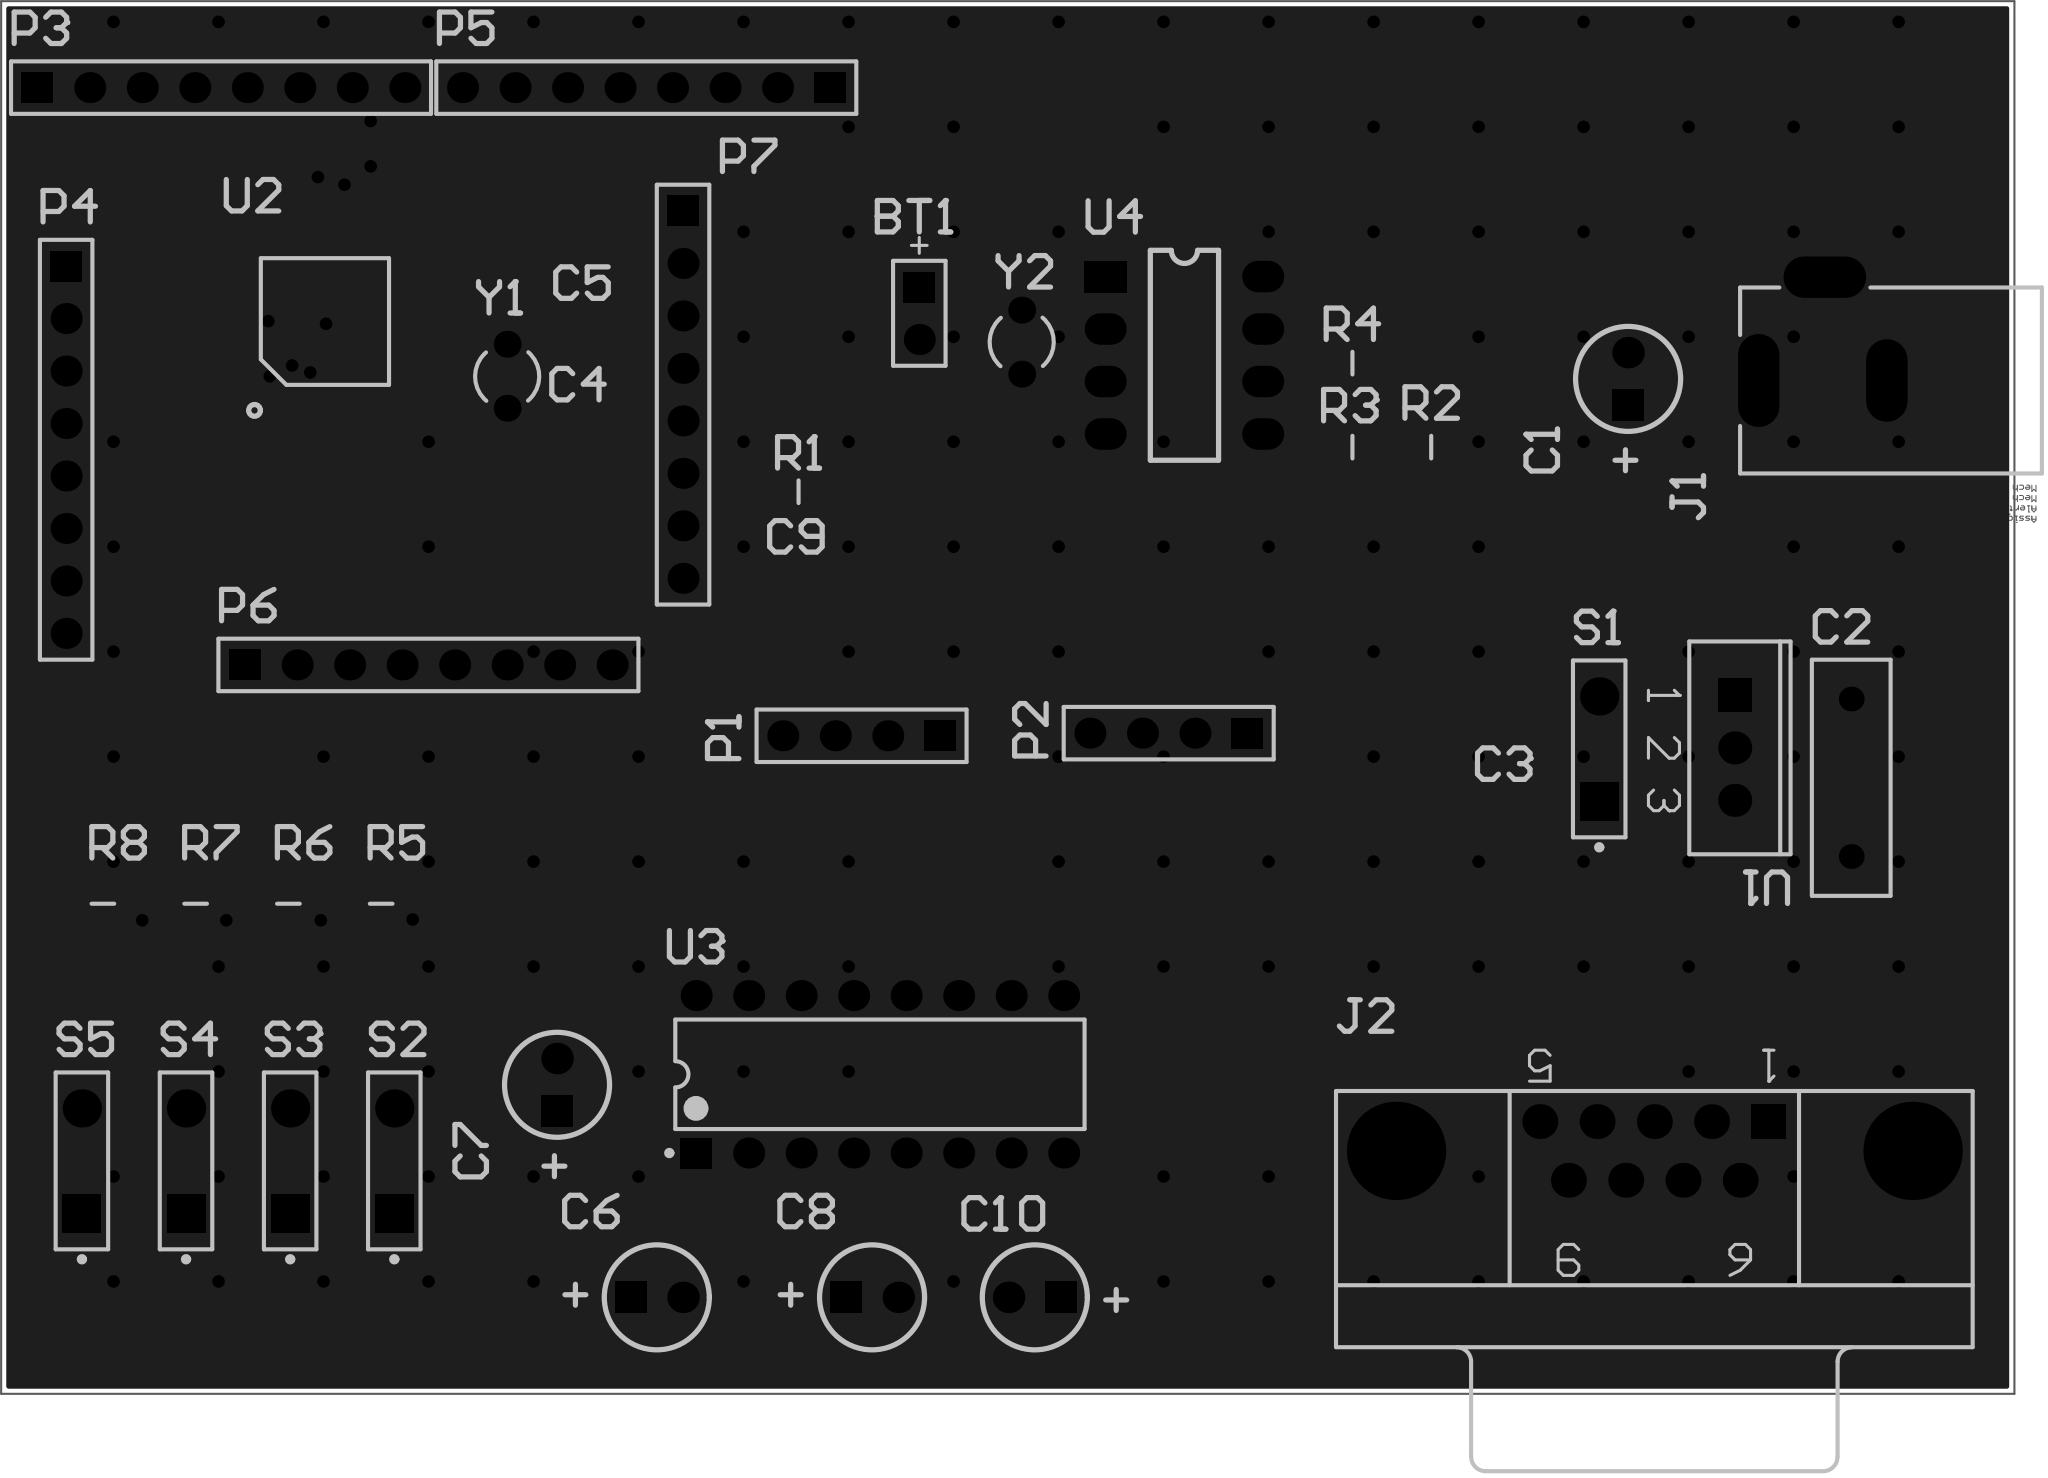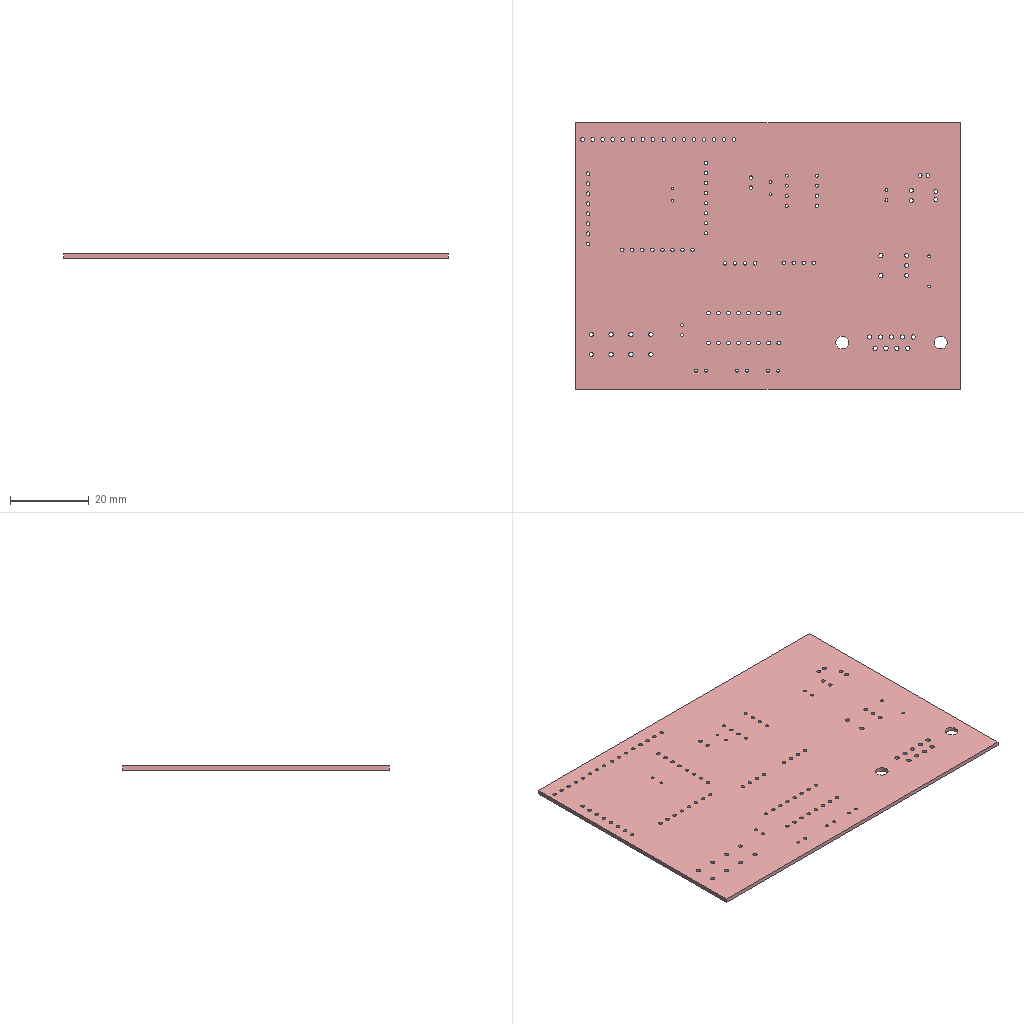Circuit board layout | Altium Designer | box 97.4 x 67.4 x 1.1 mm
Layer stack:
# Altium Designer layer stack of  (unit mm; dielectric type: 0 none, 1 core, 2 prepreg, 3 surface material)
index,name,kind,layer,copper_thickness_mm,dielectric_type,dielectric_thickness_mm,dielectric_material,dielectric_constant
0,Top Paste Mask Layer,other,,,,,,
1,Top Silkscreen Layer,other,,,,,,
2,Top Solder Mask Layer,dielectric,,,3,0.0102,Solder Resist,3.5
3,Top Layer,copper,Top Layer,0.0356,,,,
4,SUBSTRATE1,dielectric,,,3,0.32,FR-4,4.8
5,SUBSTRATE2,dielectric,,,3,0.32,FR-4,4.8
6,SUBSTRATE3,dielectric,,,3,0.32,FR-4,4.8
7,Bottom Layer,copper,Bottom Layer,0.0356,,,,
8,Bottom Solder Mask Layer,dielectric,,,3,0.0102,Solder Resist,3.5
9,Bottom Silkscreen Layer,other,,,,,,
10,Bottom Paste Mask Layer,other,,,,,,
# drill layer pairs: low layer,high layer
drill_pair,Top Layer,Bottom Layer
Part placement:
Designator,Comment,Layer,Footprint,Center-X(mm),Center-Y(mm),Rotation
Y2,XTAL,TopLayer,R38,130.937,136.652,180
Y1,XTAL,TopLayer,R38,106.045,135.001,0
U4,DS1302,TopLayer,DIP-8,138.811,136.017,0
U3,MAX232ACPE,TopLayer,PE16A,124.079,101.219,90
U2,STC12C5A60S2,TopLayer,TQFP-44,97.302,137.696,0
U1,MC7805BT,TopLayer,221A-04,165.434,117.017,270
S5,SW-PB,TopLayer,SPST-2,85.471,97.028,90
S4,SW-PB,TopLayer,SPST-2,90.509,97.028,90
S3,SW-PB,TopLayer,SPST-2,95.546,97.028,90
S2,SW-PB,TopLayer,SPST-2,100.584,97.028,90
S1,SW-SPST,TopLayer,SPST-2,158.877,116.967,90
R8,Res2,TopLayer,6-0805_L,86.487,109.474,90
R7,Res2,TopLayer,6-0805_L,90.974,109.474,90
R6,Res2,TopLayer,6-0805_L,95.462,109.474,90
R5,Res2,TopLayer,6-0805_L,99.949,109.474,90
R4,Res2,TopLayer,6-0805_L,146.939,135.636,180
R3,Res2,TopLayer,6-0805_L,146.939,131.572,0
R2,Res2,TopLayer,6-0805_L,150.749,131.572,180
R1,Res2,TopLayer,6-0805_L,120.142,129.413,180
P7,PIN4,TopLayer,HDR1X8,114.554,134.112,270
P6,PIN3,TopLayer,HDR1X8,102.235,121.031,0
P5,PIN2,TopLayer,HDR1X8,112.776,148.971,180
P4,PIN1,TopLayer,HDR1X8,84.709,131.445,270
P3,PIN0,TopLayer,HDR1X8,92.202,148.971,0
P2,POWER,TopLayer,HDR1X4,138.049,117.729,180
P1,DEBUG,TopLayer,HDR1X4,123.19,117.602,180
J2,D Connector 9,TopLayer,DSUB1.385-2H9,161.544,97.511,180
J1,PWR2.5,TopLayer,KLD-0202,169.693,136.672,180
C10,Cap Pol1,TopLayer,RB2.54-5.08,131.572,90.424,180
C9,Cap,TopLayer,C0805,120.015,125.095,0
C8,Cap Pol1,TopLayer,RB2.54-5.08,123.698,90.424,0
C7,Cap Pol1,TopLayer,RB2.54-5.08,108.458,100.711,90
C6,Cap Pol1,TopLayer,RB2.54-5.08,113.284,90.424,0
C5,Cap,TopLayer,C0805,109.601,137.16,0
C4,Cap,TopLayer,C0805,109.474,132.461,0
C3,Cap,TopLayer,C0805,154.385,114.477,0
C2,Cap,TopLayer,RAD-0.3,171.069,115.57,90
C1,Cap Pol1,TopLayer,RB2.54-5.08,160.274,134.874,90
BT1,Battery,TopLayer,BAT-2,125.984,138.049,270
Pad and via stacks:
# Altium Designer via and pad stacks of  (unit mm). Each distinct definition once, with the count of objects using it.
# via: kind,start_layer,end_layer,hole_mm,diameter_mm,mode(0 simple;1 top-mid-bottom;2 full stack),diameter_per_layer,count,example_net
# pad: kind,layer,hole_mm,hole_type(0 round;1 square;2 slot),plating,top_size,top_shape(1 round;2 rect;3 octagon;9 rounded rect),mid_size,bottom_size,mode,footprint,size_per_layer,count,example
pad,Multi-Layer,0.7,0,plated,1.3x1.3,1,1.3x1.3,1.3x1.3,0,R38,,4,Y2.1
pad,Multi-Layer,0.8128,0,plated,2.032x1.524,1,2.032x1.524,2.032x1.524,0,DIP-8,,7,U4.3
pad,Multi-Layer,0.8128,0,plated,2.032x1.524,2,2.032x1.524,2.032x1.524,0,DIP-8,,1,U4.1
pad,Multi-Layer,0.9,0,plated,1.5x1.5,1,1.5x1.5,1.5x1.5,0,PE16A,,15,U3.9
pad,Multi-Layer,0.9,0,plated,1.5x1.5,2,1.5x1.5,1.5x1.5,0,PE16A,,1,U3.1
pad,Multi-Layer,1,0,plated,1.6x1.6,2,1.6x1.6,1.6x1.6,0,221A-04,,1,U1.1
pad,Multi-Layer,1,0,plated,1.6x1.6,1,1.6x1.6,1.6x1.6,0,221A-04,,2,U1.2
pad,Multi-Layer,1.1,0,plated,1.85x1.85,2,1.85x1.85,1.85x1.85,0,SPST-2,,5,S5.1
pad,Multi-Layer,1.1,0,plated,1.85x1.85,1,1.85x1.85,1.85x1.85,0,SPST-2,,5,S5.2
pad,Multi-Layer,0.9,0,plated,1.5x1.5,2,1.5x1.5,1.5x1.5,0,HDR1X8,,5,P7.1
pad,Multi-Layer,0.9,0,plated,1.5x1.5,1,1.5x1.5,1.5x1.5,0,HDR1X8,,35,P7.2
pad,Multi-Layer,0.9,0,plated,1.5x1.5,1,1.5x1.5,1.5x1.5,0,HDR1X4,,6,P2.4
pad,Multi-Layer,0.9,0,plated,1.5x1.5,2,1.5x1.5,1.5x1.5,0,HDR1X4,,2,P2.1
pad,Multi-Layer,3.26,0,plated,4.76x4.76,1,4.76x4.76,4.76x4.76,0,DSUB1.385-2H9,,2,J2.11
pad,Multi-Layer,1.09,0,plated,1.69x1.69,2,1.69x1.69,1.69x1.69,0,DSUB1.385-2H9,,1,J2.1
pad,Multi-Layer,1.09,0,plated,1.69x1.69,1,1.69x1.69,1.69x1.69,0,DSUB1.385-2H9,,8,J2.6
pad,Multi-Layer,0,0,plated,2x4.5,1,2x4.5,2x4.5,0,KLD-0202,,1,J1.1
pad,Multi-Layer,0,0,plated,2x4,1,2x4,2x4,0,KLD-0202,,1,J1.2
pad,Multi-Layer,0,0,plated,4x2,1,4x2,4x2,0,KLD-0202,,1,J1.3
pad,Multi-Layer,1,0,plated,1.5x1.5,1,1.5x1.5,1.5x1.5,0,KLD-0202,,6,J1.1B
pad,Multi-Layer,0.762,0,plated,1.524x1.524,2,1.524x1.524,1.524x1.524,0,RB2.54-5.08,,5,C10.1
pad,Multi-Layer,0.762,0,plated,1.524x1.524,1,1.524x1.524,1.524x1.524,0,RB2.54-5.08,,5,C10.2
pad,Multi-Layer,0.7,0,plated,1.2x1.2,1,1.2x1.2,1.2x1.2,0,RAD-0.3,,2,C2.2
pad,Multi-Layer,0.9,0,plated,1.5x1.5,1,1.5x1.5,1.5x1.5,0,BAT-2,,1,BT1.2
pad,Multi-Layer,0.9,0,plated,1.5x1.5,2,1.5x1.5,1.5x1.5,0,BAT-2,,1,BT1.1
pad,Top Layer,0,0,plated,0.22x1.4,2,0.22x1.4,0.22x1.4,0,TQFP-44,,1,U2.1
pad,Top Layer,0,0,plated,0.22x1.4,1,0.22x1.4,0.22x1.4,0,TQFP-44,,43,U2.2
pad,Top Layer,0,0,plated,1.3x1,2,1.3x1,1.3x1,0,6-0805_L,,16,R8.2
pad,Top Layer,0,0,plated,1.4x1.1,2,1.4x1.1,1.4x1.1,0,C0805,,8,C9.2
via,Top Layer,Bottom Layer,0.3048,0.61,0,,161,GND
via,Top Layer,Bottom Layer,0.3048,0.6096,0,,13,P0_1
Copper pours:
name,layer,net,type(0 solid;1 hatched;2 none)
Top Layer-GND,Top Layer,GND,0
Bottom Layer-GND,Bottom Layer,GND,0
Design rules, without the lines most boards share:
# Altium Designer design rules of  (exported by Altium Designer, unit mm)
# columns: name | kind | enabled | priority | scope1 | scope2 | descriptor | typed fields (field=value)
Plane_innerPlane | 0 | disabled | 1 | All | All | Clearance Constraint (Gap=6mil) (Disabled)(All),(All) | gap=0.1524
Plane_innerPlane_1 | 63 | disabled | 1 | All | All | Board Clearance Constraint (Gap=0mil) (Disabled)(All) |
Copper_copperRegion | 0 | disabled | 2 | All | All | Clearance Constraint (Gap=6mil) (Disabled)(All),(All) | gap=0.1524
Copper_copperRegion_1 | 63 | disabled | 2 | All | All | Board Clearance Constraint (Gap=0mil) (Disabled)(All) |
safeClearance | 0 | enabled | 3 | All | All | Clearance Constraint (Gap=6mil) (All),(All) | gap=0.1524
safeClearance_1 | 63 | enabled | 3 | All | All | Board Clearance Constraint (Gap=0mil) (All) |
HoleToHoleClearance | 52 | enabled | 1 | All | All | Hole To Hole Clearance (Gap=10mil) (All),(All) | gap=0.254
trackWidth | 2 | enabled | 1 | All | All | Width Constraint (Min=5mil) (Max=100mil) (Preferred=10mil) (All) |
viaSize | 11 | enabled | 1 | All | All | Routing Via (MinHoleWidth=11.811mil) (MaxHoleWidth=236.22mil) (PreferredHoleWidth=12.008mil) (MinWidth=19.685mil) (MaxWidth=393.701mil) (PreferedWidth=24.016mil) (All) | via_min_hole=0.3 via_max_hole=6 via_preferred_diameter=0.61 via_preferred_hole=0.305